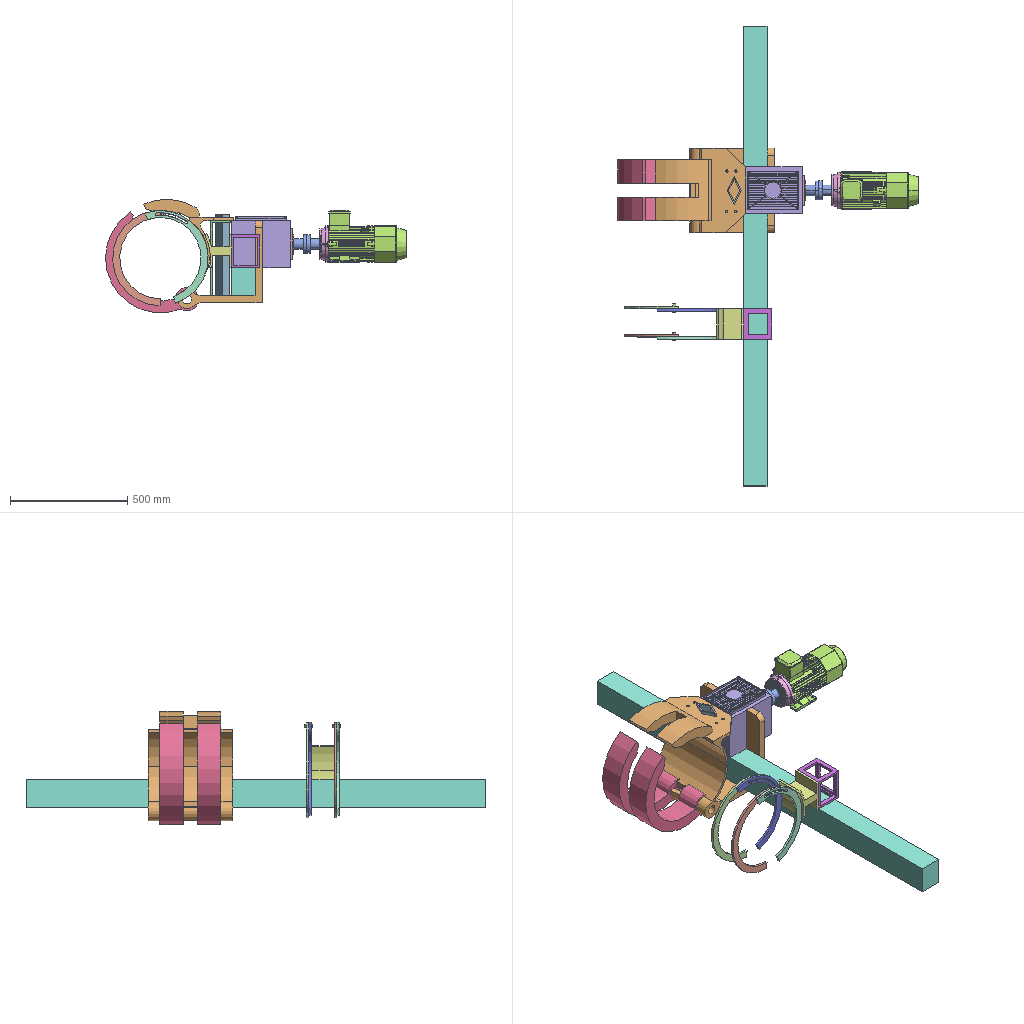Assembly | SolidWorks | 27 different items | 27 placed | box 1282 x 1959 x 482 mm
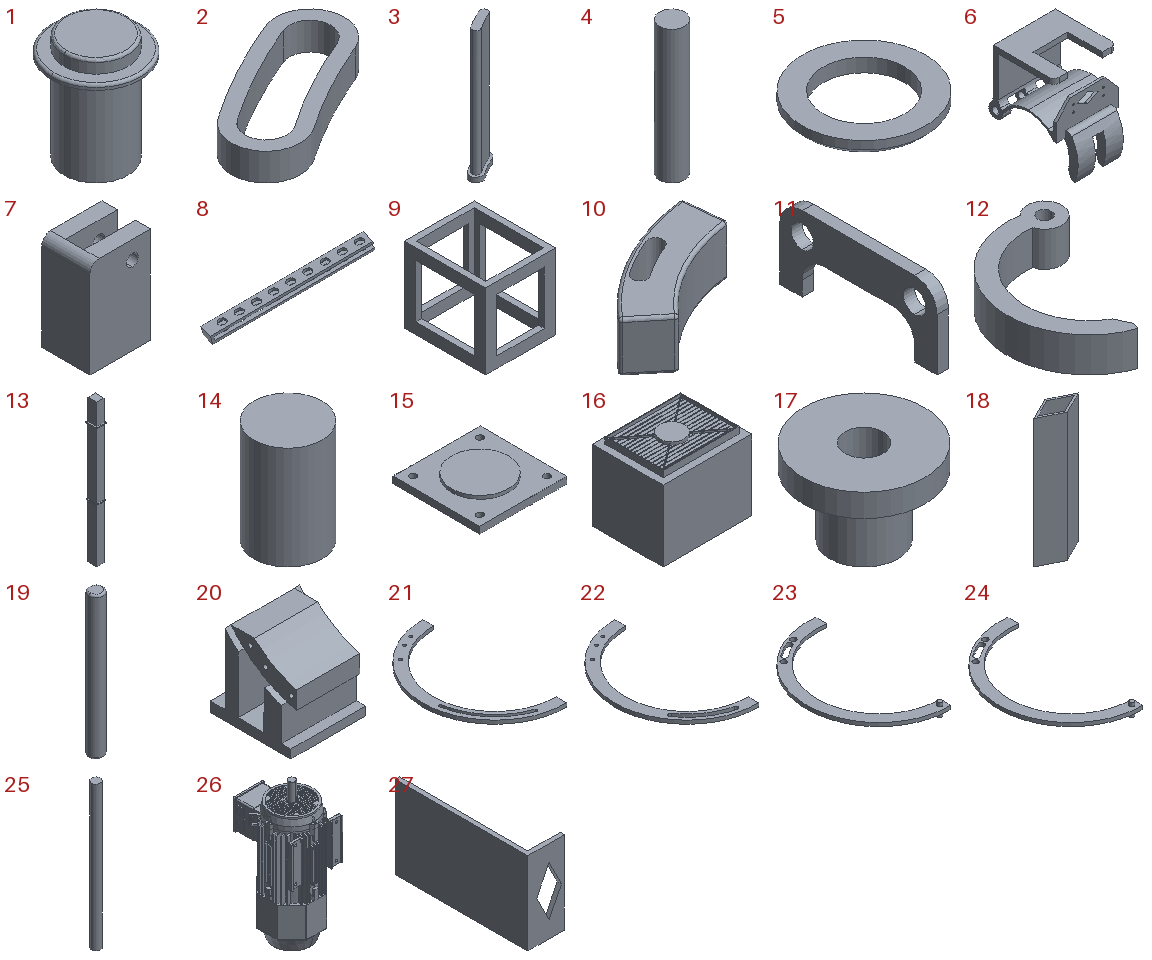Parts list (item | quantity | size | volume | features):
1 | x1 | 35 x 35 x 42 mm | 21519 mm3 | features ICE 2, Extrusion 1, Fillet 1
2 | x1 | 60.075 x 44.074 x 10 mm | 7142 mm3 | features Extrusion 1
3 | x1 | 60.075 x 44.074 x 260 mm | 209087 mm3 | features Extrusion 1, ICE 1
4 | x1 | 30 x 30 x 160 mm | 113097 mm3 | features Extrusion 1
5 | x1 | 45.387 x 45.387 x 5 mm | 4279 mm3 | features Chamfer 1, Extrusion 1
6 | x1 | 360 x 465.197 x 503.516 mm | 10385107 mm3 | features Cut 8, ICE 6, Fillet 5, BossThin 2, Chamfer 1, Extrusion 1, HoleWzd 1
7 | x1 | 99.912 x 80 x 160 mm | 851721 mm3 | features Cut 2, Extrusion 1, Fillet 1
8 | x1 | 460.11 x 161.654 x 152.871 mm | 274628 mm3 | features Cut 2, ExtruThin 1
9 | x1 | 119.912 x 140 x 130 mm | 285373 mm3 | features Cut 2, Extrusion 1
10 | x1 | 139.612 x 99.182 x 50 mm | 253889 mm3 | features Cut 2, Extrusion 1, Fillet 1
11 | x1 | 15 x 210 x 100 mm | 181294 mm3 | features Cut 1, Extrusion 1
12 | x1 | 353.552 x 466.663 x 100 mm | 3649409 mm3 | features BossThin 1, Chamfer 1, Cut 1, Extrusion 1
13 | x1 | 139.912 x 160 x 1959 mm | 23636005 mm3 | features Cut 2, ICE 2, Extrusion 1
14 | x1 | 25 x 25 x 38 mm | 18653 mm3 | features Extrusion 1
15 | x1 | 130 x 130 x 15 mm | 194231 mm3 | features Cut 1, Extrusion 1, ICE 1
16 | x1 | 250 x 200 x 218 mm | 2929125 mm3 | features ICE 3, BossThin 2, Cut 2, CutThin 1, Extrusion 1, LPattern 1
17 | x1 | 80 x 80 x 55 mm | 112017 mm3 | features Cut 1, Extrusion 1, ICE 1
18 | x1 | 120 x 60 x 348 mm | 423391 mm3 | features Cut 1, Extrusion 1
19 | x1 | 40 x 40 x 400 mm | 501382 mm3 | features Extrusion 1, Fillet 1
20 | x1 | 130 x 140 x 140 mm | 1223723 mm3 | features Cut 4, Extrusion 1, ICE 1
21 | x1 | 203.295 x 406.59 x 10 mm | 159244 mm3 | features Cut 3, Extrusion 1
22 | x1 | 203.295 x 406.59 x 10 mm | 159222 mm3 | features Cut 3, Extrusion 1
23 | x1 | 227.579 x 406.59 x 36 mm | 176233 mm3 | features Cut 1, Extrusion 1, ICE 1
24 | x1 | 227.579 x 406.59 x 36 mm | 176026 mm3 | features Cut 1, Extrusion 1, ICE 1
25 | x1 | 8 x 8 x 130 mm | 6535 mm3 | features Extrusion 1
26 | x1 | 160 x 225 x 425 mm | 6896935 mm3 | features ICE 39, Fillet 12, MirrorPattern 12, CirPattern 5, LPattern 3, Revolution 3, Chamfer 1, Dome 1, Extrusion 1, LibraryFeature 1, PLine 1, RevCut 1, Scale 1
27 | x1 | 87.761 x 320 x 200 mm | 759523 mm3 | features Cut 1, ExtruThin 1